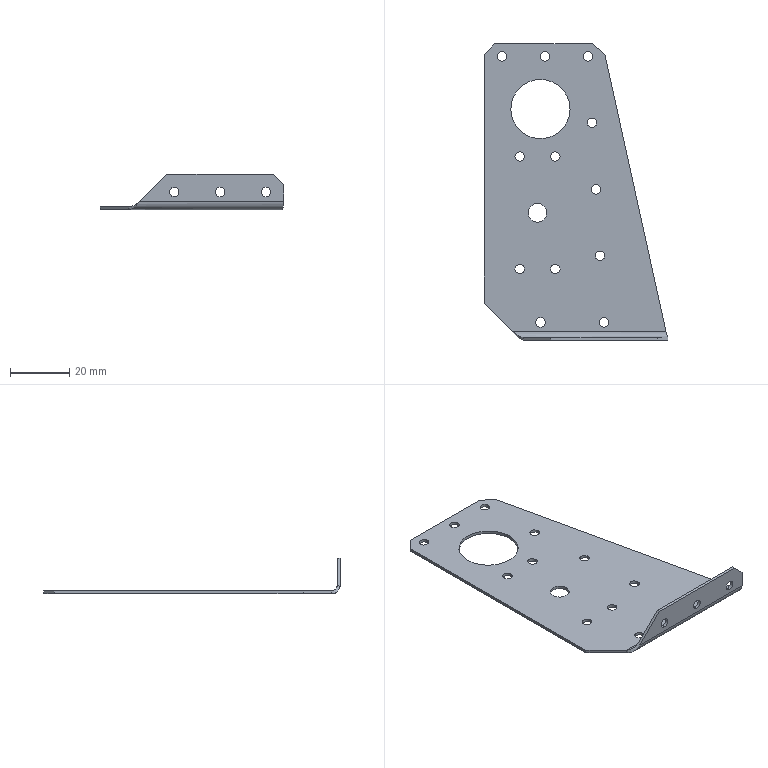Part | SolidWorks | features BaseBody 1 | 1 solid | 52 faces | box 62 x 100 x 12 mm | volume 4982 mm3 | cylinder 36 | plane 14 | spline 2 | commonest cylinder face diameters 3.2 x30 6.35 x2 20 x2 3.66 x1 5.66 x1